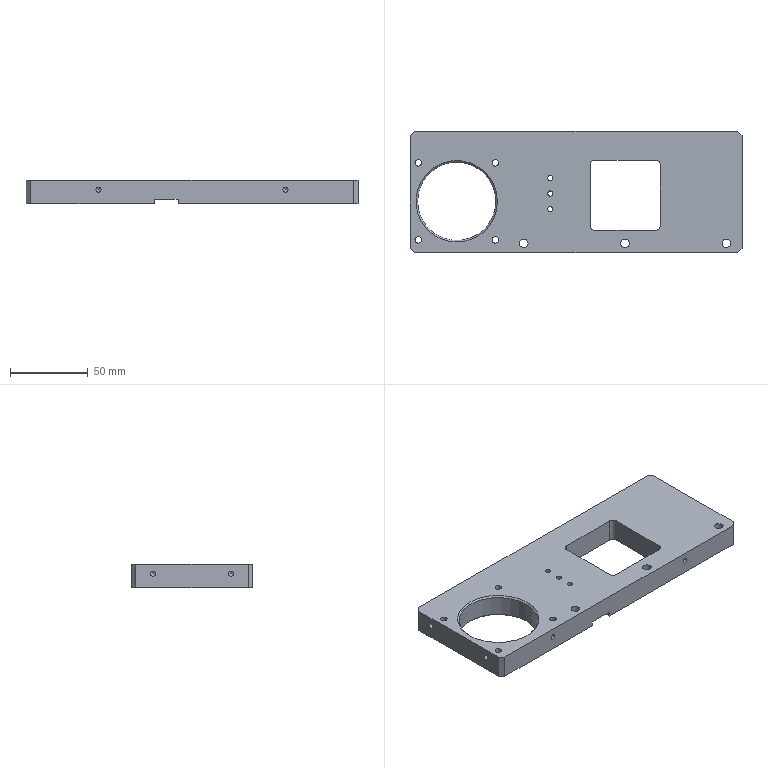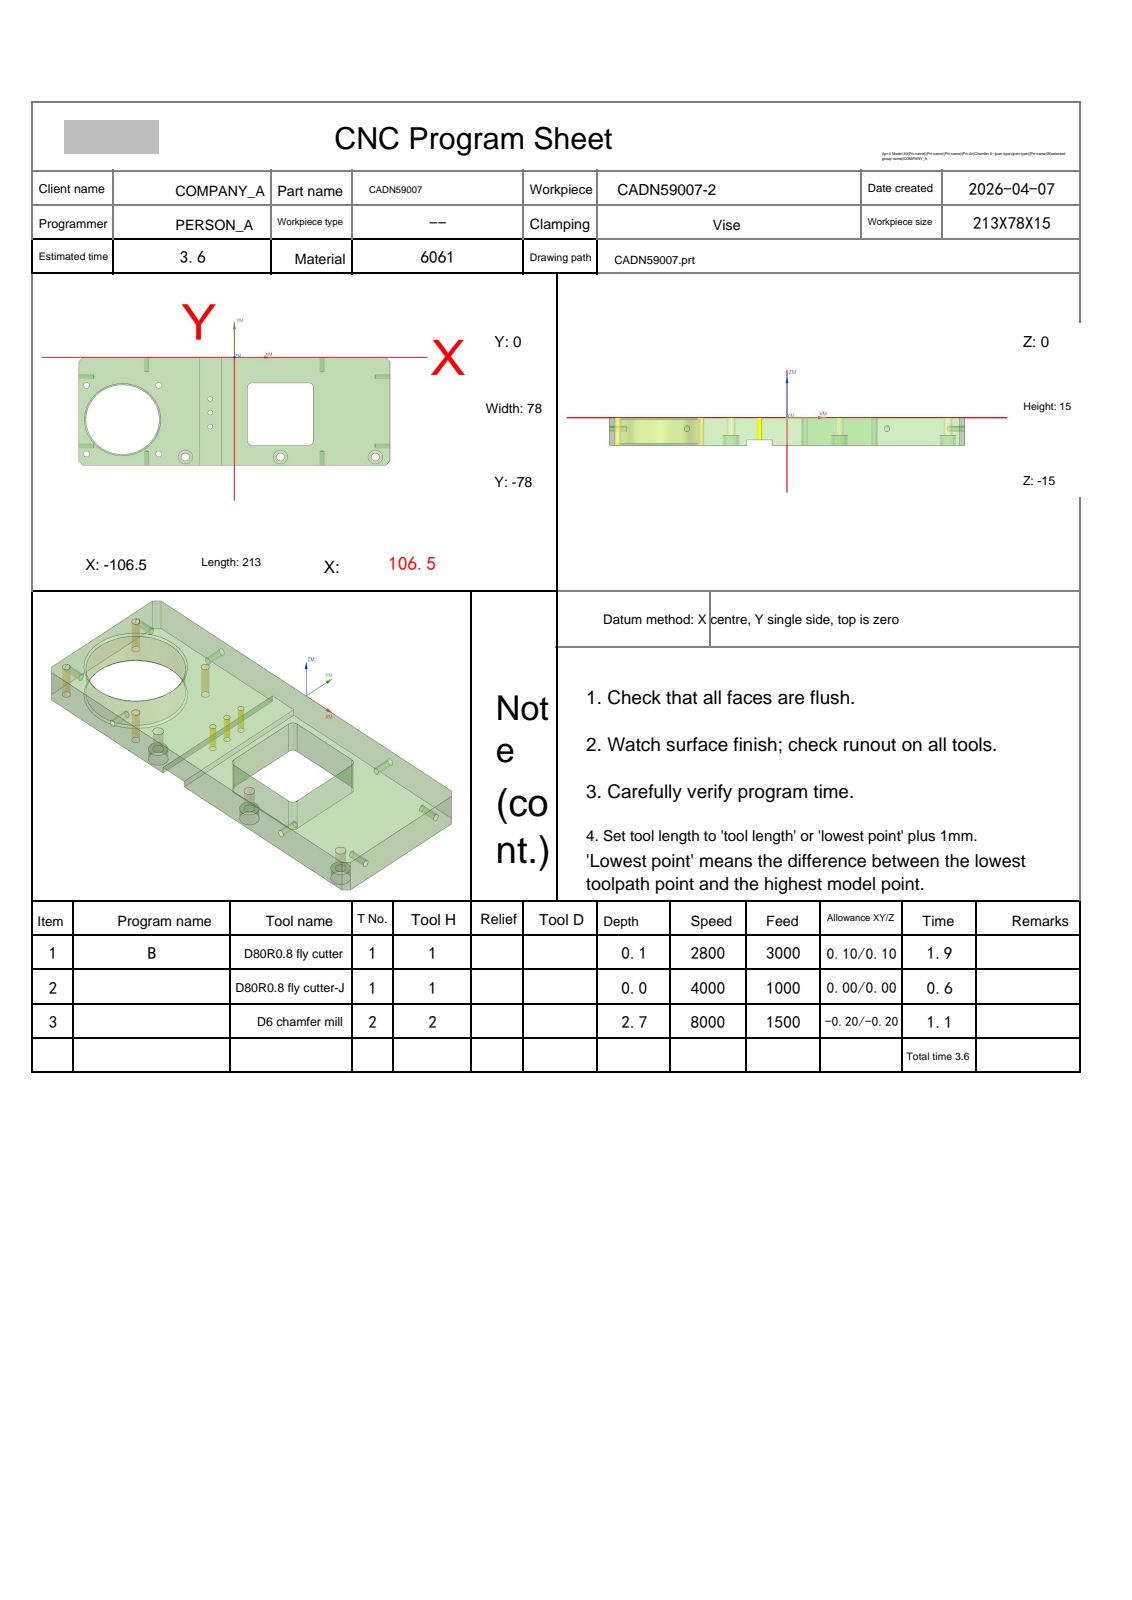NC program | NX | posted by the shop | part box 213 x 78 x 15 mm
Whole program:
%
O0001
(Machine time: 4.22 MIN)
(===Total Tool:2===)
(T1=D80R0.8 fly cutter D=80.  R=0.8  D-  H01 Z=0.    )
(T2=D6 chamfer mill   D=6.   R=0.   D-  H02 Z=-2.7  )
G80 G90 G17 G49 G40
G91 G28 Z0
M01
N1 T01 M06
(D80R0.8 fly cutter  D=80. R=0.8 H=01 ce=0.10 di=0.10)
G00 G90 G54 X-158.597 Y-23.903 M03 S2800
G43 H01 Z20.
M08
Z6.011
G01 Z4.011 F3000.
X-146.597
X139.397
G02 X146.597 Y-31.103 I0.0 J-7.2
G01 Y-38.737
G02 X138.597 Y-46.737 I-8. J0.0
G01 X-146.597
X-158.597
Z6.011
G00 Y-23.903
Z5.522
G01 Z3.522
X-146.597
X139.397
G02 X146.597 Y-31.103 I0.0 J-7.2
G01 Y-38.737
G02 X138.597 Y-46.737 I-8. J0.0
G01 X-146.597
X-158.597
Z5.522
G00 Y-23.903
Z5.033
G01 Z3.033
X-146.597
X139.397
G02 X146.597 Y-31.103 I0.0 J-7.2
G01 Y-38.737
G02 X138.597 Y-46.737 I-8. J0.0
G01 X-146.597
X-158.597
Z5.033
G00 Y-23.903
Z4.544
G01 Z2.544
X-146.597
X139.397
G02 X146.597 Y-31.103 I0.0 J-7.2
G01 Y-38.737
G02 X138.597 Y-46.737 I-8. J0.0
G01 X-146.597
X-158.597
Z4.544
G00 Y-23.903
Z4.056
G01 Z2.056
X-146.597
X139.397
G02 X146.597 Y-31.103 I0.0 J-7.2
G01 Y-38.737
G02 X138.597 Y-46.737 I-8. J0.0
G01 X-146.597
X-158.597
Z4.056
G00 Y-23.903
Z3.567
G01 Z1.567
X-146.597
X139.397
G02 X146.597 Y-31.103 I0.0 J-7.2
G01 Y-38.737
G02 X138.597 Y-46.737 I-8. J0.0
G01 X-146.597
X-158.597
Z3.567
G00 Y-23.903
Z3.078
G01 Z1.078
X-146.597
X139.397
G02 X146.597 Y-31.103 I0.0 J-7.2
G01 Y-38.737
G02 X138.597 Y-46.737 I-8. J0.0
G01 X-146.597
X-158.597
Z3.078
G00 Y-23.903
Z2.589
G01 Z.589
X-146.597
X139.397
G02 X146.597 Y-31.103 I0.0 J-7.2
G01 Y-38.737
G02 X138.597 Y-46.737 I-8. J0.0
G01 X-146.597
X-158.597
Z2.589
G00 Y-23.903
Z2.1
G01 Z.1
X-146.597
X139.397
G02 X146.597 Y-31.103 I0.0 J-7.2
G01 Y-38.737
G02 X138.597 Y-46.737 I-8. J0.0
G01 X-146.597
X-158.597
Z2.1
G00 Z20.
G91 G28 Z0.0
M05
M09
G91 G28 Z0.0
M01
N2 T01 M06
(D80R0.8 fly cutter-J  D=80. R=0.8 H=01 ce=0.00 di=0.00)
G00 G90 G54 X-158.499 Y-24.001 M03 S4000
G43 H01 Z20.
M08
Z2.
G01 Z0.0 F1000.
X-146.499
X139.299
G02 X146.499 Y-31.201 I0.0 J-7.2
G01 Y-38.639
G02 X138.499 Y-46.639 I-8. J0.0
G01 X-146.499
X-158.499
Z2.
G00 Z20.
G91 G28 Z0.0
M05
M09
G91 G28 Z0.0
M01
N3 T02 M06
(D6 chamfer mill  D=6. R=0. H=02 ce=-0.20 di=0.00)
G00 G90 G54 X18.159 Y-19.3 M03 S7000
G43 H02 Z20.
M08
Z2.5
G01 X11.885 Z.217 F1500.
X11.565 Y-19.34 Z.099
X11.254 Y-19.427 Z-.018
X10.959 Y-19.558 Z-.136
X10.687 Y-19.731 Z-.253
X10.442 Y-19.942 Z-.371
X10.231 Y-20.187 Z-.488
X10.058 Y-20.459 Z-.606
X9.927 Y-20.754 Z-.723
X9.84 Y-21.065 Z-.841
X9.8 Y-21.385 Z-.958
Y-21.5 Z-1.
Y-60.5
G03 X12. Y-62.7 I2.2 J0.0
G01 X51.
G03 X53.2 Y-60.5 I0.0 J2.2
G01 Y-21.5
G03 X51. Y-19.3 I-2.2 J0.0
G01 X12.
G03 X9.8 Y-21.5 I0.0 J-2.2
G01 Y-22.
Z1.5
G00 Z20.
X-54.026 Y-54.367
Z2.5
G01 X-53.767 Y-53.735 Z2.251
X-53.406 Y-52.729 Z1.862
X-53.089 Y-51.708 Z1.473
X-52.817 Y-50.674 Z1.084
X-52.591 Y-49.63 Z.695
X-52.411 Y-48.576 Z.306
X-52.277 Y-47.516 Z-.083
X-52.19 Y-46.45 Z-.472
X-52.15 Y-45.382 Z-.861
Y-45. Z-1.
G03 X-76.5 Y-20.65 I-24.35 J0.0
X-100.85 Y-45. I0.0 J-24.35
X-76.5 Y-69.35 I24.35 J0.0
X-52.15 Y-45. I0.0 J24.35
X-52.155 Y-44.5 I-24.35 J0.0
G01 Z1.5
G00 Z20.
G00 G90 X-16.5 Y-50. M03 S8000
Z20.
G98 G81 X-16.5 Y-50. Z-2.2 R3. F1000.
Y-40.
Y-30.
G80
G00 Z20.
G00 G90 X-51.751 Y-20.251 M03 S8000
Z20.
G98 G81 X-51.751 Y-20.251 Z-2.7 R3. F1000.
X-101.249
Y-69.749
X-51.751
G80
G00 Z20.
G00 G90 X-.386 Y1.227 M03 S6500
Z20.
Z.172
G01 Z-1.2 F1500.
G03 X-.1 Y1.027 I1.286 J1.532
G01 X-.054 Y.997
X0.0 Y1.
X103.5
X103.759 Y.966
X104. Y.866
X104.207 Y.707
X107.207 Y-2.293
X107.366 Y-2.5
X107.466 Y-2.741
X107.5 Y-3.
Y-75.
X107.466 Y-75.259
X107.366 Y-75.5
X107.207 Y-75.707
X104.207 Y-78.707
X104. Y-78.866
X103.759 Y-78.966
X103.5 Y-79.
X-103.5
X-103.759 Y-78.966
X-104. Y-78.866
X-104.207 Y-78.707
X-107.207 Y-75.707
X-107.366 Y-75.5
X-107.466 Y-75.259
X-107.5 Y-75.
Y-3.
X-107.466 Y-2.741
X-107.366 Y-2.5
X-107.207 Y-2.293
X-104.207 Y.707
X-104. Y.866
X-103.759 Y.966
X-103.5 Y1.
X0.0
X.054 Y.997
X.1 Y1.027
G03 X.386 Y1.227 I-1. J1.732
G01 Z.172
G00 Z10.
X-102.174 Y-19.839
Z.32
G01 Z-1.2
G03 X-102.335 Y-20.149 I1.687 J-1.075
G01 X-102.359 Y-20.198
X-102.349 Y-20.251
G03 X-101.249 Y-21.351 I1.1 J0.0
X-100.149 Y-20.251 I0.0 J1.1
X-101.249 Y-19.151 I-1.1 J0.0
X-102.349 Y-20.251 I0.0 J-1.1
G01 X-102.359 Y-20.305
X-102.335 Y-20.354
G03 X-102.174 Y-20.663 I1.848 J.765
G01 Z.32
G00 Z10.
X-52.677 Y-19.839
Z.32
G01 Z-1.2
G03 X-52.838 Y-20.149 I1.687 J-1.075
G01 X-52.861 Y-20.198
X-52.851 Y-20.251
G03 X-51.751 Y-21.351 I1.1 J0.0
X-50.651 Y-20.251 I0.0 J1.1
X-51.751 Y-19.151 I-1.1 J0.0
X-52.851 Y-20.251 I0.0 J-1.1
G01 X-52.861 Y-20.305
X-52.838 Y-20.354
G03 X-52.677 Y-20.663 I1.848 J.765
G01 Z.32
G00 Z10.
X-102.174 Y-69.337
Z.32
G01 Z-1.2
G03 X-102.335 Y-69.646 I1.687 J-1.075
G01 X-102.359 Y-69.695
X-102.349 Y-69.749
G03 X-101.249 Y-70.849 I1.1 J0.0
X-100.149 Y-69.749 I0.0 J1.1
X-101.249 Y-68.649 I-1.1 J0.0
X-102.349 Y-69.749 I0.0 J-1.1
G01 X-102.359 Y-69.802
X-102.335 Y-69.851
G03 X-102.174 Y-70.161 I1.848 J.765
G01 Z.32
G00 Z10.
X-52.677 Y-69.337
Z.32
G01 Z-1.2
G03 X-52.838 Y-69.646 I1.687 J-1.075
G01 X-52.861 Y-69.695
X-52.851 Y-69.749
G03 X-51.751 Y-70.849 I1.1 J0.0
X-50.651 Y-69.749 I0.0 J1.1
X-51.751 Y-68.649 I-1.1 J0.0
X-52.851 Y-69.749 I0.0 J-1.1
G01 X-52.861 Y-69.802
X-52.838 Y-69.851
G03 X-52.677 Y-70.161 I1.848 J.765
G01 Z.32
G00 Z10.
X-31.935 Y-72.407
Z.27
G01 Z-1.2
G03 X-31.766 Y-72.102 I-1.658 J1.118
G01 X-31.741 Y-72.054
X-31.75 Y-72.
G03 X-33.5 Y-70.25 I-1.75 J0.0
X-35.25 Y-72. I0.0 J-1.75
X-33.5 Y-73.75 I1.75 J0.0
X-31.75 Y-72. I0.0 J1.75
G01 X-31.741 Y-71.946
X-31.766 Y-71.898
G03 X-31.935 Y-71.593 I-1.827 J-.813
G01 Z.27
G00 Z10.
X-16.006 Y-50.419
Z.405
G01 Z-1.2
G03 X-15.859 Y-50.103 I-1.732 J1.
G01 X-15.838 Y-50.053
X-15.85 Y-50.
G03 X-16.5 Y-49.35 I-.65 J0.0
X-17.15 Y-50. I0.0 J-.65
X-16.5 Y-50.65 I.65 J0.0
X-15.85 Y-50. I0.0 J.65
G01 X-15.838 Y-49.947
X-15.859 Y-49.897
G03 X-16.006 Y-49.581 I-1.879 J-.684
G01 Z.405
G00 Z2.55
Y-40.419
Z.405
G01 Z-1.2
G03 X-15.859 Y-40.103 I-1.732 J1.
G01 X-15.838 Y-40.053
X-15.85 Y-40.
G03 X-16.5 Y-39.35 I-.65 J0.0
X-17.15 Y-40. I0.0 J-.65
X-16.5 Y-40.65 I.65 J0.0
X-15.85 Y-40. I0.0 J.65
G01 X-15.838 Y-39.947
X-15.859 Y-39.897
G03 X-16.006 Y-39.581 I-1.879 J-.684
G01 Z.405
G00 Z2.55
Y-30.419
Z.405
G01 Z-1.2
G03 X-15.859 Y-30.103 I-1.732 J1.
G01 X-15.838 Y-30.053
X-15.85 Y-30.
G03 X-16.5 Y-29.35 I-.65 J0.0
X-17.15 Y-30. I0.0 J-.65
X-16.5 Y-30.65 I.65 J0.0
X-15.85 Y-30. I0.0 J.65
G01 X-15.838 Y-29.947
X-15.859 Y-29.897
G03 X-16.006 Y-29.581 I-1.879 J-.684
G01 Z.405
G00 Z10.
X10.227 Y-40.614
Z.172
G01 Z-1.2
G03 X10.027 Y-40.9 I1.532 J-1.286
G01 X9.997 Y-40.946
X10. Y-41.
Y-60.5
G03 X12. Y-62.5 I2. J0.0
G01 X51.
G03 X53. Y-60.5 I0.0 J2.
G01 Y-21.5
G03 X51. Y-19.5 I-2. J0.0
G01 X12.
G03 X10. Y-21.5 I0.0 J-2.
G01 Y-41.
X9.997 Y-41.054
X10.027 Y-41.1
G03 X10.227 Y-41.386 I1.732 J1.
G01 Z.172
G00 Z10.
X33.065 Y-72.407
Z.27
G01 Z-1.2
G03 X33.234 Y-72.102 I-1.658 J1.118
G01 X33.259 Y-72.054
X33.25 Y-72.
G03 X31.5 Y-70.25 I-1.75 J0.0
X29.75 Y-72. I0.0 J-1.75
X31.5 Y-73.75 I1.75 J0.0
X33.25 Y-72. I0.0 J1.75
G01 X33.259 Y-71.946
X33.234 Y-71.898
G03 X33.065 Y-71.593 I-1.827 J-.813
G01 Z.27
G00 Z10.
X98.065 Y-72.407
Z.27
G01 Z-1.2
G03 X98.234 Y-72.102 I-1.658 J1.118
G01 X98.259 Y-72.054
X98.25 Y-72.
G03 X96.5 Y-70.25 I-1.75 J0.0
X94.75 Y-72. I0.0 J-1.75
X96.5 Y-73.75 I1.75 J0.0
X98.25 Y-72. I0.0 J1.75
G01 X98.259 Y-71.946
X98.234 Y-71.898
G03 X98.065 Y-71.593 I-1.827 J-.813
G01 Z.27
G00 Z20.
G00 G90 X-99.719 Y-43.8 M03 S6500
Z20.
Z-.2
G01 Z-1.7 F1500.
X-99.75
G03 X-100.95 Y-45. I0.0 J-1.2
X-76.5 Y-69.45 I24.45 J0.0
X-52.05 Y-45. I0.0 J24.45
X-76.5 Y-20.55 I-24.45 J0.0
X-100.95 Y-45. I0.0 J-24.45
X-100.947 Y-45.4 I24.45 J0.0
X-99.747 Y-46.58 I1.2 J.02
G01 X-99.727
X-99.696
Z-.2
G00 Z20.
M05
M09
G91 G28 Z0.0
G91 G28 Y0.0
M30
%